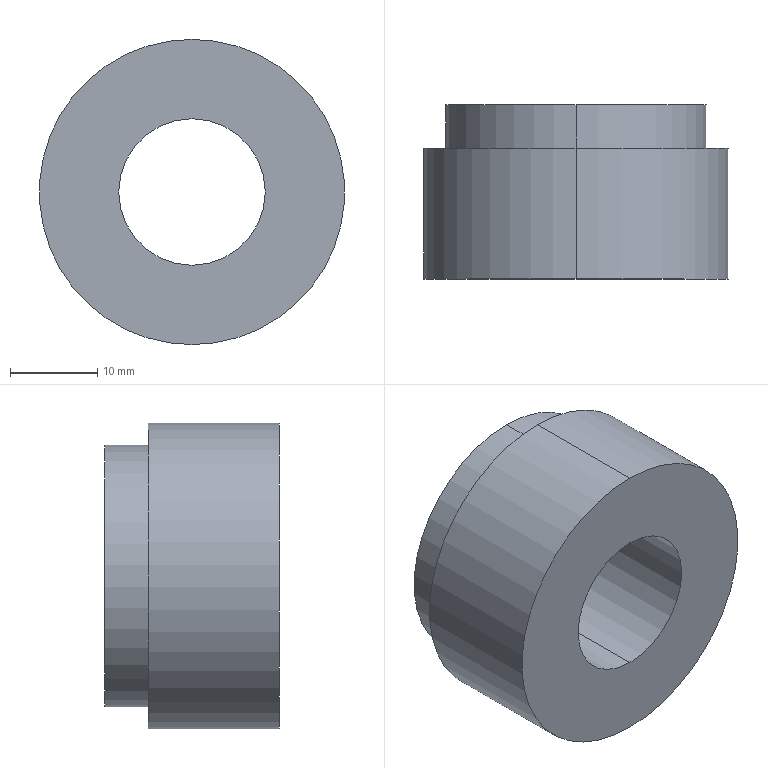Part | SolidWorks | features ICE 2, Extrusion 1 | 1 solid | 9 faces | box 35 x 20 x 35 mm | volume 13533 mm3 | cylinder 6 | plane 3 | commonest cylinder face diameters 16.8 x2 30 x2 35 x2
STEP:
#1=CARTESIAN_POINT('',(0.,0.,-8.4));
#2=VERTEX_POINT('',#1);
#3=CARTESIAN_POINT('',(0.,0.,8.4));
#4=VERTEX_POINT('',#3);
#5=CARTESIAN_POINT('',(0.,0.,0.));
#6=DIRECTION('',(0.,1.,0.));
#7=DIRECTION('',(0.,0.,1.));
#8=AXIS2_PLACEMENT_3D('',#5,#6,#7);
#9=CIRCLE('',#8,8.4);
#10=EDGE_CURVE('',#2,#4,#9,.T.);
#11=ORIENTED_EDGE('',*,*,#10,.F.);
#12=CARTESIAN_POINT('',(0.,20.,-8.4));
#13=VERTEX_POINT('',#12);
#14=CARTESIAN_POINT('',(0.,0.,-8.4));
#15=DIRECTION('',(0.,1.,0.));
#16=VECTOR('',#15,1000.);
#17=LINE('',#14,#16);
#18=EDGE_CURVE('',#2,#13,#17,.T.);
#19=ORIENTED_EDGE('',*,*,#18,.T.);
#20=CARTESIAN_POINT('',(0.,20.,8.4));
#21=VERTEX_POINT('',#20);
#22=CARTESIAN_POINT('',(0.,20.,0.));
#23=DIRECTION('',(0.,1.,0.));
#24=DIRECTION('',(0.,0.,1.));
#25=AXIS2_PLACEMENT_3D('',#22,#23,#24);
#26=CIRCLE('',#25,8.4);
#27=EDGE_CURVE('',#13,#21,#26,.T.);
#28=ORIENTED_EDGE('',*,*,#27,.T.);
#29=CARTESIAN_POINT('',(0.,0.,8.4));
#30=DIRECTION('',(0.,1.,0.));
#31=VECTOR('',#30,1000.);
#32=LINE('',#29,#31);
#33=EDGE_CURVE('',#4,#21,#32,.T.);
#34=ORIENTED_EDGE('',*,*,#33,.F.);
#35=EDGE_LOOP('',(#11,#19,#28,#34));
#36=FACE_OUTER_BOUND('',#35,.T.);
#37=CARTESIAN_POINT('',(0.,0.,0.));
#38=DIRECTION('',(0.,1.,0.));
#39=DIRECTION('',(0.,0.,1.));
#40=AXIS2_PLACEMENT_3D('',#37,#38,#39);
#41=CYLINDRICAL_SURFACE('',#40,8.4);
#42=ADVANCED_FACE('',(#36),#41,.F.);
#43=CARTESIAN_POINT('',(0.,20.,15.));
#44=VERTEX_POINT('',#43);
#45=CARTESIAN_POINT('',(0.,20.,-15.));
#46=VERTEX_POINT('',#45);
#47=CARTESIAN_POINT('',(0.,20.,0.));
#48=DIRECTION('',(0.,1.,0.));
#49=DIRECTION('',(0.,0.,1.));
#50=AXIS2_PLACEMENT_3D('',#47,#48,#49);
#51=CIRCLE('',#50,15.);
#52=EDGE_CURVE('',#44,#46,#51,.T.);
#53=ORIENTED_EDGE('',*,*,#52,.F.);
#54=CARTESIAN_POINT('',(0.,15.,15.));
#55=VERTEX_POINT('',#54);
#56=CARTESIAN_POINT('',(0.,20.,15.));
#57=DIRECTION('',(0.,-1.,0.));
#58=VECTOR('',#57,1000.);
#59=LINE('',#56,#58);
#60=EDGE_CURVE('',#44,#55,#59,.T.);
#61=ORIENTED_EDGE('',*,*,#60,.T.);
#62=CARTESIAN_POINT('',(0.,15.,-15.));
#63=VERTEX_POINT('',#62);
#64=CARTESIAN_POINT('',(0.,15.,0.));
#65=DIRECTION('',(0.,1.,0.));
#66=DIRECTION('',(0.,0.,1.));
#67=AXIS2_PLACEMENT_3D('',#64,#65,#66);
#68=CIRCLE('',#67,15.);
#69=EDGE_CURVE('',#55,#63,#68,.T.);
#70=ORIENTED_EDGE('',*,*,#69,.T.);
#71=CARTESIAN_POINT('',(0.,20.,-15.));
#72=DIRECTION('',(0.,-1.,0.));
#73=VECTOR('',#72,1000.);
#74=LINE('',#71,#73);
#75=EDGE_CURVE('',#46,#63,#74,.T.);
#76=ORIENTED_EDGE('',*,*,#75,.F.);
#77=EDGE_LOOP('',(#53,#61,#70,#76));
#78=FACE_OUTER_BOUND('',#77,.T.);
#79=CARTESIAN_POINT('',(0.,20.,0.));
#80=DIRECTION('',(0.,-1.,0.));
#81=DIRECTION('',(0.,0.,-1.));
#82=AXIS2_PLACEMENT_3D('',#79,#80,#81);
#83=CYLINDRICAL_SURFACE('',#82,15.);
#84=ADVANCED_FACE('',(#78),#83,.T.);
#85=CARTESIAN_POINT('',(0.,15.,17.5));
#86=VERTEX_POINT('',#85);
#87=CARTESIAN_POINT('',(0.,15.,-17.5));
#88=VERTEX_POINT('',#87);
#89=CARTESIAN_POINT('',(0.,15.,0.));
#90=DIRECTION('',(0.,1.,0.));
#91=DIRECTION('',(0.,0.,1.));
#92=AXIS2_PLACEMENT_3D('',#89,#90,#91);
#93=CIRCLE('',#92,17.5);
#94=EDGE_CURVE('',#86,#88,#93,.T.);
#95=ORIENTED_EDGE('',*,*,#94,.F.);
#96=CARTESIAN_POINT('',(0.,0.,17.5));
#97=VERTEX_POINT('',#96);
#98=CARTESIAN_POINT('',(0.,15.,17.5));
#99=DIRECTION('',(0.,-1.,0.));
#100=VECTOR('',#99,1000.);
#101=LINE('',#98,#100);
#102=EDGE_CURVE('',#86,#97,#101,.T.);
#103=ORIENTED_EDGE('',*,*,#102,.T.);
#104=CARTESIAN_POINT('',(0.,0.,-17.5));
#105=VERTEX_POINT('',#104);
#106=CARTESIAN_POINT('',(0.,0.,0.));
#107=DIRECTION('',(0.,1.,0.));
#108=DIRECTION('',(0.,0.,1.));
#109=AXIS2_PLACEMENT_3D('',#106,#107,#108);
#110=CIRCLE('',#109,17.5);
#111=EDGE_CURVE('',#97,#105,#110,.T.);
#112=ORIENTED_EDGE('',*,*,#111,.T.);
#113=CARTESIAN_POINT('',(0.,15.,-17.5));
#114=DIRECTION('',(0.,-1.,0.));
#115=VECTOR('',#114,1000.);
#116=LINE('',#113,#115);
#117=EDGE_CURVE('',#88,#105,#116,.T.);
#118=ORIENTED_EDGE('',*,*,#117,.F.);
#119=EDGE_LOOP('',(#95,#103,#112,#118));
#120=FACE_OUTER_BOUND('',#119,.T.);
#121=CARTESIAN_POINT('',(0.,15.,0.));
#122=DIRECTION('',(0.,-1.,0.));
#123=DIRECTION('',(0.,0.,-1.));
#124=AXIS2_PLACEMENT_3D('',#121,#122,#123);
#125=CYLINDRICAL_SURFACE('',#124,17.5);
#126=ADVANCED_FACE('',(#120),#125,.T.);
#127=ORIENTED_EDGE('',*,*,#102,.F.);
#128=CARTESIAN_POINT('',(0.,15.,0.));
#129=DIRECTION('',(0.,1.,0.));
#130=DIRECTION('',(0.,0.,1.));
#131=AXIS2_PLACEMENT_3D('',#128,#129,#130);
#132=CIRCLE('',#131,17.5);
#133=EDGE_CURVE('',#88,#86,#132,.T.);
#134=ORIENTED_EDGE('',*,*,#133,.F.);
#135=ORIENTED_EDGE('',*,*,#117,.T.);
#136=CARTESIAN_POINT('',(0.,0.,0.));
#137=DIRECTION('',(0.,1.,0.));
#138=DIRECTION('',(0.,0.,1.));
#139=AXIS2_PLACEMENT_3D('',#136,#137,#138);
#140=CIRCLE('',#139,17.5);
#141=EDGE_CURVE('',#105,#97,#140,.T.);
#142=ORIENTED_EDGE('',*,*,#141,.T.);
#143=EDGE_LOOP('',(#127,#134,#135,#142));
#144=FACE_OUTER_BOUND('',#143,.T.);
#145=CARTESIAN_POINT('',(0.,15.,0.));
#146=DIRECTION('',(0.,-1.,0.));
#147=DIRECTION('',(0.,0.,-1.));
#148=AXIS2_PLACEMENT_3D('',#145,#146,#147);
#149=CYLINDRICAL_SURFACE('',#148,17.5);
#150=ADVANCED_FACE('',(#144),#149,.T.);
#151=CARTESIAN_POINT('',(0.,15.,0.));
#152=DIRECTION('',(0.,1.,0.));
#153=DIRECTION('',(0.,0.,1.));
#154=AXIS2_PLACEMENT_3D('',#151,#152,#153);
#155=CIRCLE('',#154,15.);
#156=EDGE_CURVE('',#63,#55,#155,.T.);
#157=ORIENTED_EDGE('',*,*,#156,.F.);
#158=ORIENTED_EDGE('',*,*,#69,.F.);
#159=EDGE_LOOP('',(#157,#158));
#160=FACE_BOUND('',#159,.T.);
#161=ORIENTED_EDGE('',*,*,#133,.T.);
#162=ORIENTED_EDGE('',*,*,#94,.T.);
#163=EDGE_LOOP('',(#161,#162));
#164=FACE_OUTER_BOUND('',#163,.T.);
#165=CARTESIAN_POINT('',(0.,15.,0.));
#166=DIRECTION('',(0.,1.,0.));
#167=DIRECTION('',(0.,0.,1.));
#168=AXIS2_PLACEMENT_3D('',#165,#166,#167);
#169=PLANE('',#168);
#170=ADVANCED_FACE('',(#160,#164),#169,.T.);
#171=CARTESIAN_POINT('',(0.,0.,0.));
#172=DIRECTION('',(0.,1.,0.));
#173=DIRECTION('',(0.,0.,1.));
#174=AXIS2_PLACEMENT_3D('',#171,#172,#173);
#175=CIRCLE('',#174,8.4);
#176=EDGE_CURVE('',#4,#2,#175,.T.);
#177=ORIENTED_EDGE('',*,*,#176,.T.);
#178=ORIENTED_EDGE('',*,*,#10,.T.);
#179=EDGE_LOOP('',(#177,#178));
#180=FACE_BOUND('',#179,.T.);
#181=ORIENTED_EDGE('',*,*,#141,.F.);
#182=ORIENTED_EDGE('',*,*,#111,.F.);
#183=EDGE_LOOP('',(#181,#182));
#184=FACE_OUTER_BOUND('',#183,.T.);
#185=CARTESIAN_POINT('',(0.,0.,0.));
#186=DIRECTION('',(0.,1.,0.));
#187=DIRECTION('',(0.,0.,1.));
#188=AXIS2_PLACEMENT_3D('',#185,#186,#187);
#189=PLANE('',#188);
#190=ADVANCED_FACE('',(#180,#184),#189,.F.);
#191=ORIENTED_EDGE('',*,*,#60,.F.);
#192=CARTESIAN_POINT('',(0.,20.,0.));
#193=DIRECTION('',(0.,1.,0.));
#194=DIRECTION('',(0.,0.,1.));
#195=AXIS2_PLACEMENT_3D('',#192,#193,#194);
#196=CIRCLE('',#195,15.);
#197=EDGE_CURVE('',#46,#44,#196,.T.);
#198=ORIENTED_EDGE('',*,*,#197,.F.);
#199=ORIENTED_EDGE('',*,*,#75,.T.);
#200=ORIENTED_EDGE('',*,*,#156,.T.);
#201=EDGE_LOOP('',(#191,#198,#199,#200));
#202=FACE_OUTER_BOUND('',#201,.T.);
#203=CARTESIAN_POINT('',(0.,20.,0.));
#204=DIRECTION('',(0.,-1.,0.));
#205=DIRECTION('',(0.,0.,-1.));
#206=AXIS2_PLACEMENT_3D('',#203,#204,#205);
#207=CYLINDRICAL_SURFACE('',#206,15.);
#208=ADVANCED_FACE('',(#202),#207,.T.);
#209=CARTESIAN_POINT('',(0.,20.,0.));
#210=DIRECTION('',(0.,1.,0.));
#211=DIRECTION('',(0.,0.,1.));
#212=AXIS2_PLACEMENT_3D('',#209,#210,#211);
#213=CIRCLE('',#212,8.4);
#214=EDGE_CURVE('',#21,#13,#213,.T.);
#215=ORIENTED_EDGE('',*,*,#214,.F.);
#216=ORIENTED_EDGE('',*,*,#27,.F.);
#217=EDGE_LOOP('',(#215,#216));
#218=FACE_BOUND('',#217,.T.);
#219=ORIENTED_EDGE('',*,*,#197,.T.);
#220=ORIENTED_EDGE('',*,*,#52,.T.);
#221=EDGE_LOOP('',(#219,#220));
#222=FACE_OUTER_BOUND('',#221,.T.);
#223=CARTESIAN_POINT('',(0.,20.,0.));
#224=DIRECTION('',(0.,1.,0.));
#225=DIRECTION('',(0.,0.,1.));
#226=AXIS2_PLACEMENT_3D('',#223,#224,#225);
#227=PLANE('',#226);
#228=ADVANCED_FACE('',(#218,#222),#227,.T.);
#229=ORIENTED_EDGE('',*,*,#18,.F.);
#230=ORIENTED_EDGE('',*,*,#176,.F.);
#231=ORIENTED_EDGE('',*,*,#33,.T.);
#232=ORIENTED_EDGE('',*,*,#214,.T.);
#233=EDGE_LOOP('',(#229,#230,#231,#232));
#234=FACE_OUTER_BOUND('',#233,.T.);
#235=CARTESIAN_POINT('',(0.,0.,0.));
#236=DIRECTION('',(0.,1.,0.));
#237=DIRECTION('',(0.,0.,1.));
#238=AXIS2_PLACEMENT_3D('',#235,#236,#237);
#239=CYLINDRICAL_SURFACE('',#238,8.4);
#240=ADVANCED_FACE('',(#234),#239,.F.);
#241=CLOSED_SHELL('',(#42,#84,#126,#150,#170,#190,#208,#228,#240));
#242=MANIFOLD_SOLID_BREP('',#241);
#243=CARTESIAN_POINT('',(0.,0.,0.));
#244=DIRECTION('',(0.,0.,1.));
#245=DIRECTION('',(1.,0.,0.));
#246=AXIS2_PLACEMENT_3D('',#243,#244,#245);
#247=(LENGTH_UNIT()NAMED_UNIT(*)SI_UNIT(.MILLI.,.METRE.));
#248=UNCERTAINTY_MEASURE_WITH_UNIT(LENGTH_MEASURE(0.00001),#247,'','');
#249=(NAMED_UNIT(*)PLANE_ANGLE_UNIT()SI_UNIT($,.RADIAN.));
#250=(NAMED_UNIT(*)SI_UNIT($,.STERADIAN.)SOLID_ANGLE_UNIT());
#251=(GEOMETRIC_REPRESENTATION_CONTEXT(3)GLOBAL_UNCERTAINTY_ASSIGNED_CONTEXT((#248))GLOBAL_UNIT_ASSIGNED_CONTEXT((#247,#249,#250))REPRESENTATION_CONTEXT('',''));
#252=ADVANCED_BREP_SHAPE_REPRESENTATION('',(#242,#246),#251);